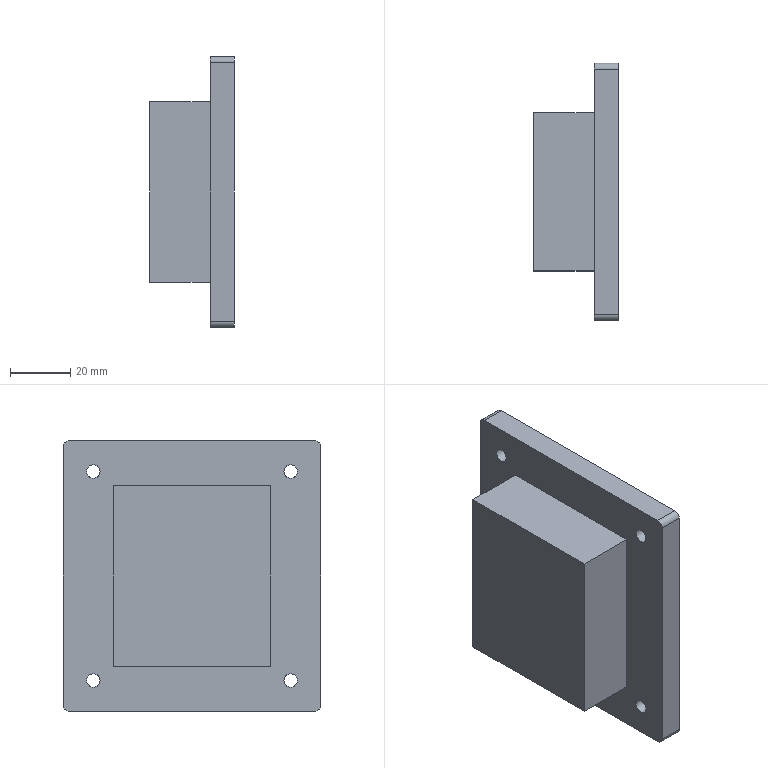Part | STEP file | 冲床-300配套压波_id306_x_t | 1 solid | 19 faces | box 28 x 85.6 x 90 mm | volume 124096 mm3 | plane 11 | cylinder 8 | commonest cylinder face diameters 4 x4 4.5 x4
STEP:
#1=CARTESIAN_POINT('',(1921.2,138.75,-655.));
#2=VERTEX_POINT('',#1);
#3=CARTESIAN_POINT('',(1921.2,191.25,-655.));
#4=VERTEX_POINT('',#3);
#5=CARTESIAN_POINT('',(1921.2,138.75,-655.));
#6=DIRECTION('',(0.,1.,0.));
#7=VECTOR('',#6,1.);
#8=LINE('',#5,#7);
#9=EDGE_CURVE('',#2,#4,#8,.T.);
#10=ORIENTED_EDGE('',*,*,#9,.T.);
#11=CARTESIAN_POINT('',(1921.2,191.25,-595.));
#12=VERTEX_POINT('',#11);
#13=CARTESIAN_POINT('',(1921.2,191.25,-655.));
#14=DIRECTION('',(0.,0.,1.));
#15=VECTOR('',#14,1.);
#16=LINE('',#13,#15);
#17=EDGE_CURVE('',#4,#12,#16,.T.);
#18=ORIENTED_EDGE('',*,*,#17,.T.);
#19=CARTESIAN_POINT('',(1921.2,138.75,-595.));
#20=VERTEX_POINT('',#19);
#21=CARTESIAN_POINT('',(1921.2,191.25,-595.));
#22=DIRECTION('',(0.,-1.,0.));
#23=VECTOR('',#22,1.);
#24=LINE('',#21,#23);
#25=EDGE_CURVE('',#12,#20,#24,.T.);
#26=ORIENTED_EDGE('',*,*,#25,.T.);
#27=CARTESIAN_POINT('',(1921.2,138.75,-595.));
#28=DIRECTION('',(0.,0.,-1.));
#29=VECTOR('',#28,1.);
#30=LINE('',#27,#29);
#31=EDGE_CURVE('',#20,#2,#30,.T.);
#32=ORIENTED_EDGE('',*,*,#31,.T.);
#33=EDGE_LOOP('',(#10,#18,#26,#32));
#34=FACE_BOUND('',#33,.T.);
#35=CARTESIAN_POINT('',(1921.2,200.1,-590.25));
#36=VERTEX_POINT('',#35);
#37=CARTESIAN_POINT('',(1921.2,197.85,-590.25));
#38=DIRECTION('',(-1.,0.,0.));
#39=DIRECTION('',(0.,1.,0.));
#40=AXIS2_PLACEMENT_3D('',#37,#38,#39);
#41=CIRCLE('',#40,2.25);
#42=EDGE_CURVE('',#36,#36,#41,.T.);
#43=ORIENTED_EDGE('',*,*,#42,.F.);
#44=EDGE_LOOP('',(#43));
#45=FACE_BOUND('',#44,.T.);
#46=CARTESIAN_POINT('',(1921.2,129.9,-590.25));
#47=VERTEX_POINT('',#46);
#48=CARTESIAN_POINT('',(1921.2,132.15,-590.25));
#49=DIRECTION('',(-1.,0.,0.));
#50=DIRECTION('',(0.,-1.,0.));
#51=AXIS2_PLACEMENT_3D('',#48,#49,#50);
#52=CIRCLE('',#51,2.25);
#53=EDGE_CURVE('',#47,#47,#52,.T.);
#54=ORIENTED_EDGE('',*,*,#53,.F.);
#55=EDGE_LOOP('',(#54));
#56=FACE_BOUND('',#55,.T.);
#57=CARTESIAN_POINT('',(1921.2,207.8,-668.));
#58=VERTEX_POINT('',#57);
#59=CARTESIAN_POINT('',(1921.2,207.8,-582.));
#60=VERTEX_POINT('',#59);
#61=CARTESIAN_POINT('',(1921.2,207.8,-670.));
#62=DIRECTION('',(0.,0.,1.));
#63=VECTOR('',#62,1.);
#64=LINE('',#61,#63);
#65=EDGE_CURVE('',#58,#60,#64,.T.);
#66=ORIENTED_EDGE('',*,*,#65,.F.);
#67=CARTESIAN_POINT('',(1921.2,205.8,-670.));
#68=VERTEX_POINT('',#67);
#69=CARTESIAN_POINT('',(1921.2,205.8,-668.));
#70=DIRECTION('',(-1.,0.,0.));
#71=DIRECTION('',(0.,0.,-1.));
#72=AXIS2_PLACEMENT_3D('',#69,#70,#71);
#73=CIRCLE('',#72,2.);
#74=EDGE_CURVE('',#58,#68,#73,.T.);
#75=ORIENTED_EDGE('',*,*,#74,.T.);
#76=CARTESIAN_POINT('',(1921.2,124.2,-670.));
#77=VERTEX_POINT('',#76);
#78=CARTESIAN_POINT('',(1921.2,122.2,-670.));
#79=DIRECTION('',(0.,1.,0.));
#80=VECTOR('',#79,1.);
#81=LINE('',#78,#80);
#82=EDGE_CURVE('',#77,#68,#81,.T.);
#83=ORIENTED_EDGE('',*,*,#82,.F.);
#84=CARTESIAN_POINT('',(1921.2,122.2,-668.));
#85=VERTEX_POINT('',#84);
#86=CARTESIAN_POINT('',(1921.2,124.2,-668.));
#87=DIRECTION('',(-1.,0.,0.));
#88=DIRECTION('',(0.,0.,-1.));
#89=AXIS2_PLACEMENT_3D('',#86,#87,#88);
#90=CIRCLE('',#89,2.);
#91=EDGE_CURVE('',#77,#85,#90,.T.);
#92=ORIENTED_EDGE('',*,*,#91,.T.);
#93=CARTESIAN_POINT('',(1921.2,122.2,-582.));
#94=VERTEX_POINT('',#93);
#95=CARTESIAN_POINT('',(1921.2,122.2,-580.));
#96=DIRECTION('',(0.,0.,-1.));
#97=VECTOR('',#96,1.);
#98=LINE('',#95,#97);
#99=EDGE_CURVE('',#94,#85,#98,.T.);
#100=ORIENTED_EDGE('',*,*,#99,.F.);
#101=CARTESIAN_POINT('',(1921.2,124.2,-580.));
#102=VERTEX_POINT('',#101);
#103=CARTESIAN_POINT('',(1921.2,124.2,-582.));
#104=DIRECTION('',(-1.,0.,0.));
#105=DIRECTION('',(0.,0.,-1.));
#106=AXIS2_PLACEMENT_3D('',#103,#104,#105);
#107=CIRCLE('',#106,2.);
#108=EDGE_CURVE('',#94,#102,#107,.T.);
#109=ORIENTED_EDGE('',*,*,#108,.T.);
#110=CARTESIAN_POINT('',(1921.2,205.8,-580.));
#111=VERTEX_POINT('',#110);
#112=CARTESIAN_POINT('',(1921.2,207.8,-580.));
#113=DIRECTION('',(0.,-1.,0.));
#114=VECTOR('',#113,1.);
#115=LINE('',#112,#114);
#116=EDGE_CURVE('',#111,#102,#115,.T.);
#117=ORIENTED_EDGE('',*,*,#116,.F.);
#118=CARTESIAN_POINT('',(1921.2,205.8,-582.));
#119=DIRECTION('',(-1.,0.,0.));
#120=DIRECTION('',(0.,0.,-1.));
#121=AXIS2_PLACEMENT_3D('',#118,#119,#120);
#122=CIRCLE('',#121,2.);
#123=EDGE_CURVE('',#111,#60,#122,.T.);
#124=ORIENTED_EDGE('',*,*,#123,.T.);
#125=EDGE_LOOP('',(#66,#75,#83,#92,#100,#109,#117,#124));
#126=FACE_BOUND('',#125,.T.);
#127=CARTESIAN_POINT('',(1921.2,200.1,-659.75));
#128=VERTEX_POINT('',#127);
#129=CARTESIAN_POINT('',(1921.2,197.85,-659.75));
#130=DIRECTION('',(-1.,0.,0.));
#131=DIRECTION('',(0.,1.,0.));
#132=AXIS2_PLACEMENT_3D('',#129,#130,#131);
#133=CIRCLE('',#132,2.25);
#134=EDGE_CURVE('',#128,#128,#133,.T.);
#135=ORIENTED_EDGE('',*,*,#134,.F.);
#136=EDGE_LOOP('',(#135));
#137=FACE_BOUND('',#136,.T.);
#138=CARTESIAN_POINT('',(1921.2,129.9,-659.75));
#139=VERTEX_POINT('',#138);
#140=CARTESIAN_POINT('',(1921.2,132.15,-659.75));
#141=DIRECTION('',(1.,0.,0.));
#142=DIRECTION('',(0.,-1.,0.));
#143=AXIS2_PLACEMENT_3D('',#140,#141,#142);
#144=CIRCLE('',#143,2.25);
#145=EDGE_CURVE('',#139,#139,#144,.T.);
#146=ORIENTED_EDGE('',*,*,#145,.T.);
#147=EDGE_LOOP('',(#146));
#148=FACE_BOUND('',#147,.T.);
#149=CARTESIAN_POINT('',(1921.2,8.,12.));
#150=DIRECTION('',(1.,0.,0.));
#151=DIRECTION('',(0.,0.,-1.));
#152=AXIS2_PLACEMENT_3D('',#149,#150,#151);
#153=PLANE('',#152);
#154=ADVANCED_FACE('',(#34,#45,#56,#126,#137,#148),#153,.F.);
#155=CARTESIAN_POINT('',(1929.2,197.85,-592.5));
#156=VERTEX_POINT('',#155);
#157=CARTESIAN_POINT('',(1929.2,197.85,-590.25));
#158=DIRECTION('',(1.,0.,0.));
#159=DIRECTION('',(0.,0.,-1.));
#160=AXIS2_PLACEMENT_3D('',#157,#158,#159);
#161=CIRCLE('',#160,2.25);
#162=EDGE_CURVE('',#156,#156,#161,.T.);
#163=ORIENTED_EDGE('',*,*,#162,.F.);
#164=EDGE_LOOP('',(#163));
#165=FACE_BOUND('',#164,.T.);
#166=CARTESIAN_POINT('',(1929.2,132.15,-592.5));
#167=VERTEX_POINT('',#166);
#168=CARTESIAN_POINT('',(1929.2,132.15,-590.25));
#169=DIRECTION('',(1.,0.,0.));
#170=DIRECTION('',(0.,0.,-1.));
#171=AXIS2_PLACEMENT_3D('',#168,#169,#170);
#172=CIRCLE('',#171,2.25);
#173=EDGE_CURVE('',#167,#167,#172,.T.);
#174=ORIENTED_EDGE('',*,*,#173,.F.);
#175=EDGE_LOOP('',(#174));
#176=FACE_BOUND('',#175,.T.);
#177=CARTESIAN_POINT('',(1929.2,124.2,-670.));
#178=VERTEX_POINT('',#177);
#179=CARTESIAN_POINT('',(1929.2,205.8,-670.));
#180=VERTEX_POINT('',#179);
#181=CARTESIAN_POINT('',(1929.2,122.2,-670.));
#182=DIRECTION('',(0.,1.,0.));
#183=VECTOR('',#182,1.);
#184=LINE('',#181,#183);
#185=EDGE_CURVE('',#178,#180,#184,.T.);
#186=ORIENTED_EDGE('',*,*,#185,.T.);
#187=CARTESIAN_POINT('',(1929.2,207.8,-668.));
#188=VERTEX_POINT('',#187);
#189=CARTESIAN_POINT('',(1929.2,205.8,-668.));
#190=DIRECTION('',(1.,0.,0.));
#191=DIRECTION('',(0.,0.,-1.));
#192=AXIS2_PLACEMENT_3D('',#189,#190,#191);
#193=CIRCLE('',#192,2.);
#194=EDGE_CURVE('',#180,#188,#193,.T.);
#195=ORIENTED_EDGE('',*,*,#194,.T.);
#196=CARTESIAN_POINT('',(1929.2,207.8,-582.));
#197=VERTEX_POINT('',#196);
#198=CARTESIAN_POINT('',(1929.2,207.8,-670.));
#199=DIRECTION('',(0.,0.,1.));
#200=VECTOR('',#199,1.);
#201=LINE('',#198,#200);
#202=EDGE_CURVE('',#188,#197,#201,.T.);
#203=ORIENTED_EDGE('',*,*,#202,.T.);
#204=CARTESIAN_POINT('',(1929.2,205.8,-580.));
#205=VERTEX_POINT('',#204);
#206=CARTESIAN_POINT('',(1929.2,205.8,-582.));
#207=DIRECTION('',(1.,0.,0.));
#208=DIRECTION('',(0.,0.,-1.));
#209=AXIS2_PLACEMENT_3D('',#206,#207,#208);
#210=CIRCLE('',#209,2.);
#211=EDGE_CURVE('',#197,#205,#210,.T.);
#212=ORIENTED_EDGE('',*,*,#211,.T.);
#213=CARTESIAN_POINT('',(1929.2,124.2,-580.));
#214=VERTEX_POINT('',#213);
#215=CARTESIAN_POINT('',(1929.2,207.8,-580.));
#216=DIRECTION('',(0.,-1.,0.));
#217=VECTOR('',#216,1.);
#218=LINE('',#215,#217);
#219=EDGE_CURVE('',#205,#214,#218,.T.);
#220=ORIENTED_EDGE('',*,*,#219,.T.);
#221=CARTESIAN_POINT('',(1929.2,122.2,-582.));
#222=VERTEX_POINT('',#221);
#223=CARTESIAN_POINT('',(1929.2,124.2,-582.));
#224=DIRECTION('',(1.,0.,0.));
#225=DIRECTION('',(0.,0.,-1.));
#226=AXIS2_PLACEMENT_3D('',#223,#224,#225);
#227=CIRCLE('',#226,2.);
#228=EDGE_CURVE('',#214,#222,#227,.T.);
#229=ORIENTED_EDGE('',*,*,#228,.T.);
#230=CARTESIAN_POINT('',(1929.2,122.2,-668.));
#231=VERTEX_POINT('',#230);
#232=CARTESIAN_POINT('',(1929.2,122.2,-580.));
#233=DIRECTION('',(0.,0.,-1.));
#234=VECTOR('',#233,1.);
#235=LINE('',#232,#234);
#236=EDGE_CURVE('',#222,#231,#235,.T.);
#237=ORIENTED_EDGE('',*,*,#236,.T.);
#238=CARTESIAN_POINT('',(1929.2,124.2,-668.));
#239=DIRECTION('',(1.,0.,0.));
#240=DIRECTION('',(0.,0.,-1.));
#241=AXIS2_PLACEMENT_3D('',#238,#239,#240);
#242=CIRCLE('',#241,2.);
#243=EDGE_CURVE('',#231,#178,#242,.T.);
#244=ORIENTED_EDGE('',*,*,#243,.T.);
#245=EDGE_LOOP('',(#186,#195,#203,#212,#220,#229,#237,#244));
#246=FACE_BOUND('',#245,.T.);
#247=CARTESIAN_POINT('',(1929.2,197.85,-662.));
#248=VERTEX_POINT('',#247);
#249=CARTESIAN_POINT('',(1929.2,197.85,-659.75));
#250=DIRECTION('',(1.,0.,0.));
#251=DIRECTION('',(0.,0.,-1.));
#252=AXIS2_PLACEMENT_3D('',#249,#250,#251);
#253=CIRCLE('',#252,2.25);
#254=EDGE_CURVE('',#248,#248,#253,.T.);
#255=ORIENTED_EDGE('',*,*,#254,.F.);
#256=EDGE_LOOP('',(#255));
#257=FACE_BOUND('',#256,.T.);
#258=CARTESIAN_POINT('',(1929.2,132.15,-662.));
#259=VERTEX_POINT('',#258);
#260=CARTESIAN_POINT('',(1929.2,132.15,-659.75));
#261=DIRECTION('',(-1.,0.,0.));
#262=DIRECTION('',(0.,0.,-1.));
#263=AXIS2_PLACEMENT_3D('',#260,#261,#262);
#264=CIRCLE('',#263,2.25);
#265=EDGE_CURVE('',#259,#259,#264,.T.);
#266=ORIENTED_EDGE('',*,*,#265,.T.);
#267=EDGE_LOOP('',(#266));
#268=FACE_BOUND('',#267,.T.);
#269=CARTESIAN_POINT('',(1929.2,8.,12.));
#270=DIRECTION('',(1.,0.,0.));
#271=DIRECTION('',(0.,0.,-1.));
#272=AXIS2_PLACEMENT_3D('',#269,#270,#271);
#273=PLANE('',#272);
#274=ADVANCED_FACE('',(#165,#176,#246,#257,#268),#273,.T.);
#275=ORIENTED_EDGE('',*,*,#99,.T.);
#276=CARTESIAN_POINT('',(1921.2,122.2,-668.));
#277=DIRECTION('',(1.,0.,0.));
#278=VECTOR('',#277,1.);
#279=LINE('',#276,#278);
#280=EDGE_CURVE('',#85,#231,#279,.T.);
#281=ORIENTED_EDGE('',*,*,#280,.T.);
#282=ORIENTED_EDGE('',*,*,#236,.F.);
#283=CARTESIAN_POINT('',(1921.2,122.2,-582.));
#284=DIRECTION('',(-1.,0.,0.));
#285=VECTOR('',#284,1.);
#286=LINE('',#283,#285);
#287=EDGE_CURVE('',#222,#94,#286,.T.);
#288=ORIENTED_EDGE('',*,*,#287,.T.);
#289=EDGE_LOOP('',(#275,#281,#282,#288));
#290=FACE_OUTER_BOUND('',#289,.T.);
#291=CARTESIAN_POINT('',(1921.2,122.2,-580.));
#292=DIRECTION('',(0.,-1.,0.));
#293=DIRECTION('',(0.,0.,-1.));
#294=AXIS2_PLACEMENT_3D('',#291,#292,#293);
#295=PLANE('',#294);
#296=ADVANCED_FACE('',(#290),#295,.T.);
#297=ORIENTED_EDGE('',*,*,#82,.T.);
#298=CARTESIAN_POINT('',(1921.2,205.8,-670.));
#299=DIRECTION('',(1.,0.,0.));
#300=VECTOR('',#299,1.);
#301=LINE('',#298,#300);
#302=EDGE_CURVE('',#68,#180,#301,.T.);
#303=ORIENTED_EDGE('',*,*,#302,.T.);
#304=ORIENTED_EDGE('',*,*,#185,.F.);
#305=CARTESIAN_POINT('',(1921.2,124.2,-670.));
#306=DIRECTION('',(-1.,0.,0.));
#307=VECTOR('',#306,1.);
#308=LINE('',#305,#307);
#309=EDGE_CURVE('',#178,#77,#308,.T.);
#310=ORIENTED_EDGE('',*,*,#309,.T.);
#311=EDGE_LOOP('',(#297,#303,#304,#310));
#312=FACE_OUTER_BOUND('',#311,.T.);
#313=CARTESIAN_POINT('',(1921.2,122.2,-670.));
#314=DIRECTION('',(0.,0.,-1.));
#315=DIRECTION('',(-1.,0.,0.));
#316=AXIS2_PLACEMENT_3D('',#313,#314,#315);
#317=PLANE('',#316);
#318=ADVANCED_FACE('',(#312),#317,.T.);
#319=ORIENTED_EDGE('',*,*,#202,.F.);
#320=CARTESIAN_POINT('',(1921.2,207.8,-668.));
#321=DIRECTION('',(-1.,0.,0.));
#322=VECTOR('',#321,1.);
#323=LINE('',#320,#322);
#324=EDGE_CURVE('',#188,#58,#323,.T.);
#325=ORIENTED_EDGE('',*,*,#324,.T.);
#326=ORIENTED_EDGE('',*,*,#65,.T.);
#327=CARTESIAN_POINT('',(1921.2,207.8,-582.));
#328=DIRECTION('',(1.,0.,0.));
#329=VECTOR('',#328,1.);
#330=LINE('',#327,#329);
#331=EDGE_CURVE('',#60,#197,#330,.T.);
#332=ORIENTED_EDGE('',*,*,#331,.T.);
#333=EDGE_LOOP('',(#319,#325,#326,#332));
#334=FACE_OUTER_BOUND('',#333,.T.);
#335=CARTESIAN_POINT('',(1921.2,207.8,-670.));
#336=DIRECTION('',(0.,1.,0.));
#337=DIRECTION('',(0.,0.,1.));
#338=AXIS2_PLACEMENT_3D('',#335,#336,#337);
#339=PLANE('',#338);
#340=ADVANCED_FACE('',(#334),#339,.T.);
#341=ORIENTED_EDGE('',*,*,#116,.T.);
#342=CARTESIAN_POINT('',(1921.2,124.2,-580.));
#343=DIRECTION('',(1.,0.,0.));
#344=VECTOR('',#343,1.);
#345=LINE('',#342,#344);
#346=EDGE_CURVE('',#102,#214,#345,.T.);
#347=ORIENTED_EDGE('',*,*,#346,.T.);
#348=ORIENTED_EDGE('',*,*,#219,.F.);
#349=CARTESIAN_POINT('',(1921.2,205.8,-580.));
#350=DIRECTION('',(-1.,0.,0.));
#351=VECTOR('',#350,1.);
#352=LINE('',#349,#351);
#353=EDGE_CURVE('',#205,#111,#352,.T.);
#354=ORIENTED_EDGE('',*,*,#353,.T.);
#355=EDGE_LOOP('',(#341,#347,#348,#354));
#356=FACE_OUTER_BOUND('',#355,.T.);
#357=CARTESIAN_POINT('',(1921.2,207.8,-580.));
#358=DIRECTION('',(0.,0.,1.));
#359=DIRECTION('',(1.,0.,0.));
#360=AXIS2_PLACEMENT_3D('',#357,#358,#359);
#361=PLANE('',#360);
#362=ADVANCED_FACE('',(#356),#361,.T.);
#363=ORIENTED_EDGE('',*,*,#254,.T.);
#364=EDGE_LOOP('',(#363));
#365=FACE_BOUND('',#364,.T.);
#366=ORIENTED_EDGE('',*,*,#134,.T.);
#367=EDGE_LOOP('',(#366));
#368=FACE_BOUND('',#367,.T.);
#369=CARTESIAN_POINT('',(1941.2,197.85,-659.75));
#370=DIRECTION('',(-1.,0.,0.));
#371=DIRECTION('',(0.,0.,1.));
#372=AXIS2_PLACEMENT_3D('',#369,#370,#371);
#373=CYLINDRICAL_SURFACE('',#372,2.25);
#374=ADVANCED_FACE('',(#365,#368),#373,.F.);
#375=ORIENTED_EDGE('',*,*,#265,.F.);
#376=EDGE_LOOP('',(#375));
#377=FACE_BOUND('',#376,.T.);
#378=ORIENTED_EDGE('',*,*,#145,.F.);
#379=EDGE_LOOP('',(#378));
#380=FACE_BOUND('',#379,.T.);
#381=CARTESIAN_POINT('',(1941.2,132.15,-659.75));
#382=DIRECTION('',(-1.,0.,0.));
#383=DIRECTION('',(0.,0.,1.));
#384=AXIS2_PLACEMENT_3D('',#381,#382,#383);
#385=CYLINDRICAL_SURFACE('',#384,2.25);
#386=ADVANCED_FACE('',(#377,#380),#385,.F.);
#387=ORIENTED_EDGE('',*,*,#173,.T.);
#388=EDGE_LOOP('',(#387));
#389=FACE_BOUND('',#388,.T.);
#390=ORIENTED_EDGE('',*,*,#53,.T.);
#391=EDGE_LOOP('',(#390));
#392=FACE_BOUND('',#391,.T.);
#393=CARTESIAN_POINT('',(1941.2,132.15,-590.25));
#394=DIRECTION('',(-1.,0.,0.));
#395=DIRECTION('',(0.,0.,1.));
#396=AXIS2_PLACEMENT_3D('',#393,#394,#395);
#397=CYLINDRICAL_SURFACE('',#396,2.25);
#398=ADVANCED_FACE('',(#389,#392),#397,.F.);
#399=ORIENTED_EDGE('',*,*,#162,.T.);
#400=EDGE_LOOP('',(#399));
#401=FACE_BOUND('',#400,.T.);
#402=ORIENTED_EDGE('',*,*,#42,.T.);
#403=EDGE_LOOP('',(#402));
#404=FACE_BOUND('',#403,.T.);
#405=CARTESIAN_POINT('',(1941.2,197.85,-590.25));
#406=DIRECTION('',(-1.,0.,0.));
#407=DIRECTION('',(0.,0.,1.));
#408=AXIS2_PLACEMENT_3D('',#405,#406,#407);
#409=CYLINDRICAL_SURFACE('',#408,2.25);
#410=ADVANCED_FACE('',(#401,#404),#409,.F.);
#411=ORIENTED_EDGE('',*,*,#17,.F.);
#412=CARTESIAN_POINT('',(1901.2,191.25,-655.));
#413=VERTEX_POINT('',#412);
#414=CARTESIAN_POINT('',(1901.2,191.25,-655.));
#415=DIRECTION('',(1.,0.,0.));
#416=VECTOR('',#415,1.);
#417=LINE('',#414,#416);
#418=EDGE_CURVE('',#413,#4,#417,.T.);
#419=ORIENTED_EDGE('',*,*,#418,.F.);
#420=CARTESIAN_POINT('',(1901.2,191.25,-595.));
#421=VERTEX_POINT('',#420);
#422=CARTESIAN_POINT('',(1901.2,191.25,-655.));
#423=DIRECTION('',(0.,0.,1.));
#424=VECTOR('',#423,1.);
#425=LINE('',#422,#424);
#426=EDGE_CURVE('',#413,#421,#425,.T.);
#427=ORIENTED_EDGE('',*,*,#426,.T.);
#428=CARTESIAN_POINT('',(1901.2,191.25,-595.));
#429=DIRECTION('',(1.,0.,0.));
#430=VECTOR('',#429,1.);
#431=LINE('',#428,#430);
#432=EDGE_CURVE('',#421,#12,#431,.T.);
#433=ORIENTED_EDGE('',*,*,#432,.T.);
#434=EDGE_LOOP('',(#411,#419,#427,#433));
#435=FACE_OUTER_BOUND('',#434,.T.);
#436=CARTESIAN_POINT('',(1901.2,191.25,-655.));
#437=DIRECTION('',(0.,1.,0.));
#438=DIRECTION('',(0.,0.,1.));
#439=AXIS2_PLACEMENT_3D('',#436,#437,#438);
#440=PLANE('',#439);
#441=ADVANCED_FACE('',(#435),#440,.T.);
#442=ORIENTED_EDGE('',*,*,#25,.F.);
#443=ORIENTED_EDGE('',*,*,#432,.F.);
#444=CARTESIAN_POINT('',(1901.2,138.75,-595.));
#445=VERTEX_POINT('',#444);
#446=CARTESIAN_POINT('',(1901.2,191.25,-595.));
#447=DIRECTION('',(0.,-1.,0.));
#448=VECTOR('',#447,1.);
#449=LINE('',#446,#448);
#450=EDGE_CURVE('',#421,#445,#449,.T.);
#451=ORIENTED_EDGE('',*,*,#450,.T.);
#452=CARTESIAN_POINT('',(1901.2,138.75,-595.));
#453=DIRECTION('',(1.,0.,0.));
#454=VECTOR('',#453,1.);
#455=LINE('',#452,#454);
#456=EDGE_CURVE('',#445,#20,#455,.T.);
#457=ORIENTED_EDGE('',*,*,#456,.T.);
#458=EDGE_LOOP('',(#442,#443,#451,#457));
#459=FACE_OUTER_BOUND('',#458,.T.);
#460=CARTESIAN_POINT('',(1901.2,191.25,-595.));
#461=DIRECTION('',(0.,0.,1.));
#462=DIRECTION('',(1.,0.,0.));
#463=AXIS2_PLACEMENT_3D('',#460,#461,#462);
#464=PLANE('',#463);
#465=ADVANCED_FACE('',(#459),#464,.T.);
#466=ORIENTED_EDGE('',*,*,#31,.F.);
#467=ORIENTED_EDGE('',*,*,#456,.F.);
#468=CARTESIAN_POINT('',(1901.2,138.75,-655.));
#469=VERTEX_POINT('',#468);
#470=CARTESIAN_POINT('',(1901.2,138.75,-595.));
#471=DIRECTION('',(0.,0.,-1.));
#472=VECTOR('',#471,1.);
#473=LINE('',#470,#472);
#474=EDGE_CURVE('',#445,#469,#473,.T.);
#475=ORIENTED_EDGE('',*,*,#474,.T.);
#476=CARTESIAN_POINT('',(1901.2,138.75,-655.));
#477=DIRECTION('',(1.,0.,0.));
#478=VECTOR('',#477,1.);
#479=LINE('',#476,#478);
#480=EDGE_CURVE('',#469,#2,#479,.T.);
#481=ORIENTED_EDGE('',*,*,#480,.T.);
#482=EDGE_LOOP('',(#466,#467,#475,#481));
#483=FACE_OUTER_BOUND('',#482,.T.);
#484=CARTESIAN_POINT('',(1901.2,138.75,-595.));
#485=DIRECTION('',(0.,-1.,0.));
#486=DIRECTION('',(0.,0.,-1.));
#487=AXIS2_PLACEMENT_3D('',#484,#485,#486);
#488=PLANE('',#487);
#489=ADVANCED_FACE('',(#483),#488,.T.);
#490=ORIENTED_EDGE('',*,*,#9,.F.);
#491=ORIENTED_EDGE('',*,*,#480,.F.);
#492=CARTESIAN_POINT('',(1901.2,138.75,-655.));
#493=DIRECTION('',(0.,1.,0.));
#494=VECTOR('',#493,1.);
#495=LINE('',#492,#494);
#496=EDGE_CURVE('',#469,#413,#495,.T.);
#497=ORIENTED_EDGE('',*,*,#496,.T.);
#498=ORIENTED_EDGE('',*,*,#418,.T.);
#499=EDGE_LOOP('',(#490,#491,#497,#498));
#500=FACE_OUTER_BOUND('',#499,.T.);
#501=CARTESIAN_POINT('',(1901.2,138.75,-655.));
#502=DIRECTION('',(0.,0.,-1.));
#503=DIRECTION('',(-1.,0.,0.));
#504=AXIS2_PLACEMENT_3D('',#501,#502,#503);
#505=PLANE('',#504);
#506=ADVANCED_FACE('',(#500),#505,.T.);
#507=ORIENTED_EDGE('',*,*,#426,.F.);
#508=ORIENTED_EDGE('',*,*,#496,.F.);
#509=ORIENTED_EDGE('',*,*,#474,.F.);
#510=ORIENTED_EDGE('',*,*,#450,.F.);
#511=EDGE_LOOP('',(#507,#508,#509,#510));
#512=FACE_OUTER_BOUND('',#511,.T.);
#513=CARTESIAN_POINT('',(1901.2,8.,12.));
#514=DIRECTION('',(1.,0.,0.));
#515=DIRECTION('',(0.,0.,-1.));
#516=AXIS2_PLACEMENT_3D('',#513,#514,#515);
#517=PLANE('',#516);
#518=ADVANCED_FACE('',(#512),#517,.F.);
#519=ORIENTED_EDGE('',*,*,#194,.F.);
#520=ORIENTED_EDGE('',*,*,#302,.F.);
#521=ORIENTED_EDGE('',*,*,#74,.F.);
#522=ORIENTED_EDGE('',*,*,#324,.F.);
#523=EDGE_LOOP('',(#519,#520,#521,#522));
#524=FACE_OUTER_BOUND('',#523,.T.);
#525=CARTESIAN_POINT('',(1921.2,205.8,-668.));
#526=DIRECTION('',(-1.,0.,0.));
#527=DIRECTION('',(0.,0.,1.));
#528=AXIS2_PLACEMENT_3D('',#525,#526,#527);
#529=CYLINDRICAL_SURFACE('',#528,2.);
#530=ADVANCED_FACE('',(#524),#529,.T.);
#531=ORIENTED_EDGE('',*,*,#243,.F.);
#532=ORIENTED_EDGE('',*,*,#280,.F.);
#533=ORIENTED_EDGE('',*,*,#91,.F.);
#534=ORIENTED_EDGE('',*,*,#309,.F.);
#535=EDGE_LOOP('',(#531,#532,#533,#534));
#536=FACE_OUTER_BOUND('',#535,.T.);
#537=CARTESIAN_POINT('',(1921.2,124.2,-668.));
#538=DIRECTION('',(-1.,0.,0.));
#539=DIRECTION('',(0.,0.,1.));
#540=AXIS2_PLACEMENT_3D('',#537,#538,#539);
#541=CYLINDRICAL_SURFACE('',#540,2.);
#542=ADVANCED_FACE('',(#536),#541,.T.);
#543=ORIENTED_EDGE('',*,*,#228,.F.);
#544=ORIENTED_EDGE('',*,*,#346,.F.);
#545=ORIENTED_EDGE('',*,*,#108,.F.);
#546=ORIENTED_EDGE('',*,*,#287,.F.);
#547=EDGE_LOOP('',(#543,#544,#545,#546));
#548=FACE_OUTER_BOUND('',#547,.T.);
#549=CARTESIAN_POINT('',(1921.2,124.2,-582.));
#550=DIRECTION('',(-1.,0.,0.));
#551=DIRECTION('',(0.,0.,1.));
#552=AXIS2_PLACEMENT_3D('',#549,#550,#551);
#553=CYLINDRICAL_SURFACE('',#552,2.);
#554=ADVANCED_FACE('',(#548),#553,.T.);
#555=ORIENTED_EDGE('',*,*,#211,.F.);
#556=ORIENTED_EDGE('',*,*,#331,.F.);
#557=ORIENTED_EDGE('',*,*,#123,.F.);
#558=ORIENTED_EDGE('',*,*,#353,.F.);
#559=EDGE_LOOP('',(#555,#556,#557,#558));
#560=FACE_OUTER_BOUND('',#559,.T.);
#561=CARTESIAN_POINT('',(1921.2,205.8,-582.));
#562=DIRECTION('',(-1.,0.,0.));
#563=DIRECTION('',(0.,0.,1.));
#564=AXIS2_PLACEMENT_3D('',#561,#562,#563);
#565=CYLINDRICAL_SURFACE('',#564,2.);
#566=ADVANCED_FACE('',(#560),#565,.T.);
#567=CLOSED_SHELL('',(#154,#274,#296,#318,#340,#362,#374,#386,#398,#410,#441,#465,#489,#506,#518,#530,#542,#554,#566));
#568=MANIFOLD_SOLID_BREP('',#567);
#569=(LENGTH_UNIT()NAMED_UNIT(*)SI_UNIT(.MILLI.,.METRE.));
#570=UNCERTAINTY_MEASURE_WITH_UNIT(LENGTH_MEASURE(0.00002),#569,'','');
#571=(NAMED_UNIT(*)PLANE_ANGLE_UNIT()SI_UNIT($,.RADIAN.));
#572=PLANE_ANGLE_MEASURE_WITH_UNIT(PLANE_ANGLE_MEASURE(0.01745),#571);
#573=DIMENSIONAL_EXPONENTS(0.,0.,0.,0.,0.,0.,0.);
#574=(CONVERSION_BASED_UNIT('DEGREE',#572)NAMED_UNIT(#573)PLANE_ANGLE_UNIT());
#575=(NAMED_UNIT(*)SI_UNIT($,.STERADIAN.)SOLID_ANGLE_UNIT());
#576=(GEOMETRIC_REPRESENTATION_CONTEXT(3)GLOBAL_UNCERTAINTY_ASSIGNED_CONTEXT((#570))GLOBAL_UNIT_ASSIGNED_CONTEXT((#569,#574,#575))REPRESENTATION_CONTEXT('',''));
#577=ADVANCED_BREP_SHAPE_REPRESENTATION('',(#568),#576);